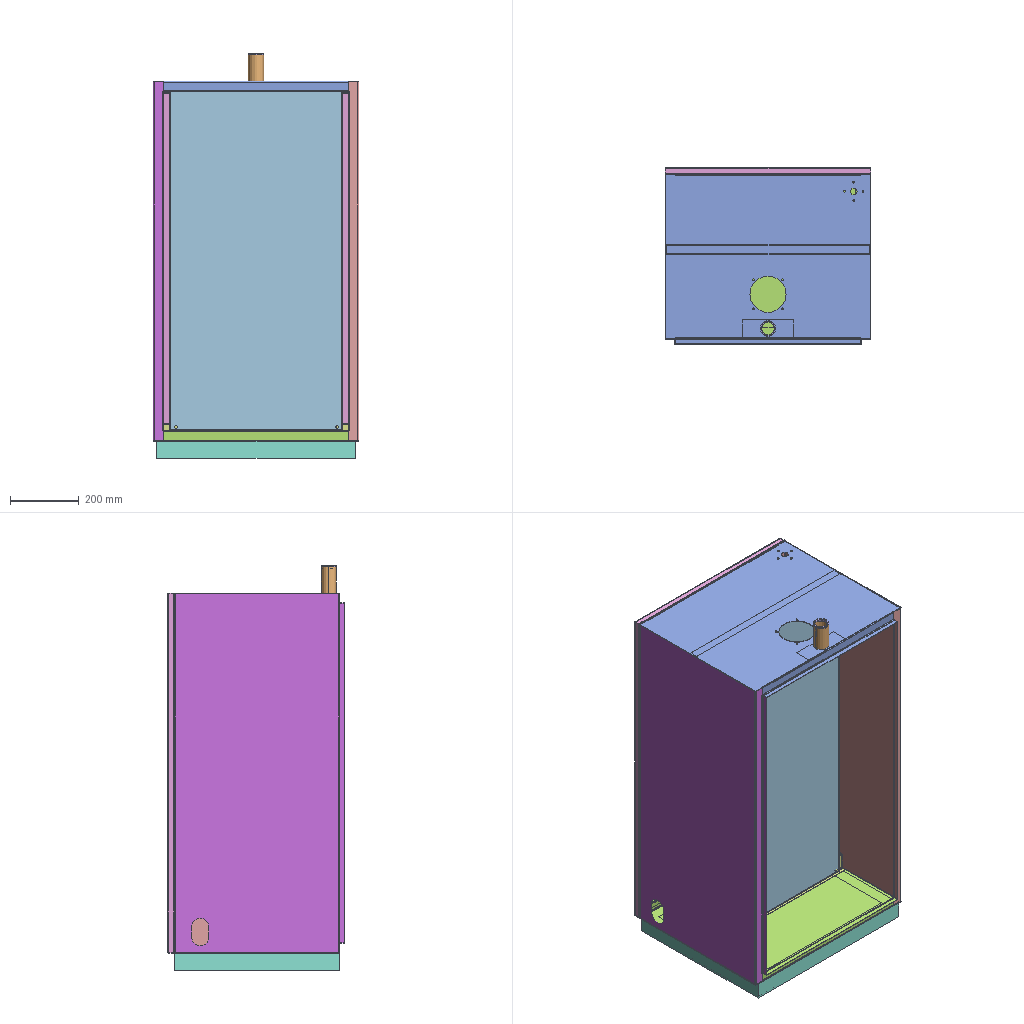Assembly | SolidWorks | 13 different items | 14 placed | box 600 x 515 x 1180 mm
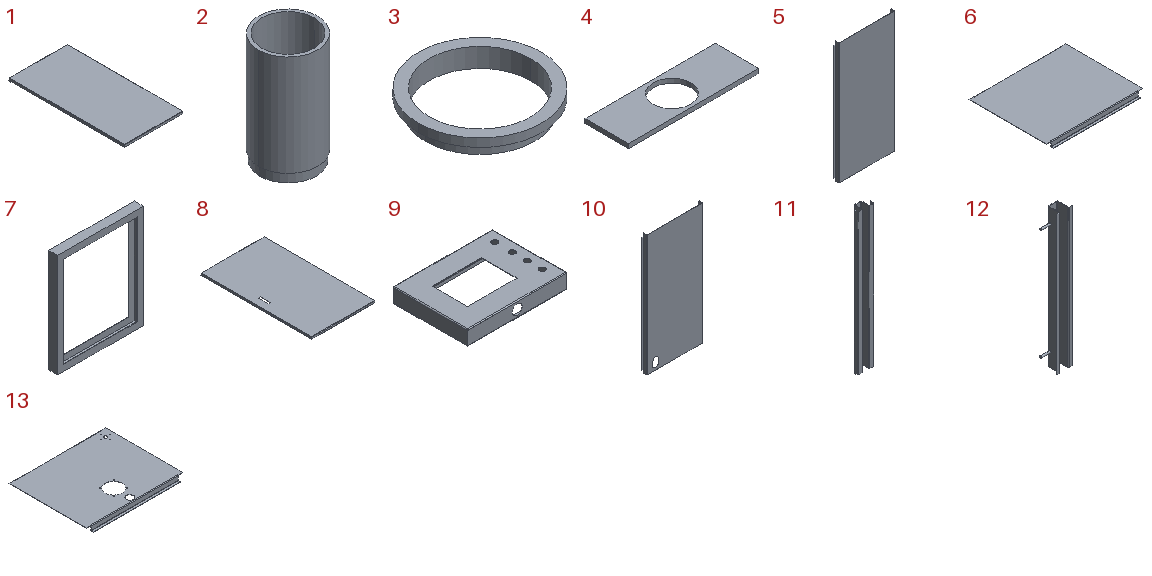Parts list (item | quantity | size | volume | features):
1 | x2 | 505 x 1000 x 25 mm | 849677 mm3 | features EdgeFlange 2, CornerFeat 1, FlatPattern 1, ICE 1, SMBaseFlange 1, SheetMetal 1
2 | x1 | 45 x 45 x 84 mm | 27071 mm3 | features Extrusion 1, ICE 1
3 | x1 | 45 x 45 x 7 mm | 2271 mm3 | features Extrusion 1, ICE 1
4 | x1 | 150 x 50 x 5 mm | 30239 mm3 | features FlatPattern 1, ICE 1, SMBaseFlange 1, SheetMetal 1
5 | x1 | 510 x 30 x 1047 mm | 882007 mm3 | features EdgeFlange 2, FlatPattern 1, SMBaseFlange 1, SheetMetal 1
6 | x1 | 600 x 510 x 30 mm | 499324 mm3 | features EdgeFlange 2, FlatPattern 1, SMBaseFlange 1, SheetMetal 1
7 | x1 | 480 x 50 x 580 mm | 907872 mm3 | features ICE 2, Extrusion 1
8 | x1 | 600 x 1050 x 20 mm | 1074617 mm3 | features EdgeFlange 2, CornerFeat 1, FlatPattern 1, ICE 1, SMBaseFlange 1, SheetMetal 1
9 | x1 | 400 x 300 x 73.5 mm | 309583 mm3 | features EdgeFlange 3, ICE 2, CornerFeat 1, FlatPattern 1, SMBaseFlange 1, SheetMetal 1
10 | x1 | 510 x 30 x 1047 mm | 876812 mm3 | features EdgeFlange 2, FlatPattern 1, ICE 1, SMBaseFlange 1, SheetMetal 1
11 | x1 | 67 x 35 x 590 mm | 137357 mm3 | features FlatPattern 1, SMBaseFlange 1, SheetMetal 1
12 | x1 | 120 x 50 x 590 mm | 149764 mm3 | features ICE 2, EdgeFlange 1, FlatPattern 1, SMBaseFlange 1, SheetMetal 1
13 | x1 | 600 x 510 x 30 mm | 483219 mm3 | features ICE 3, EdgeFlange 2, FlatPattern 1, SMBaseFlange 1, SheetMetal 1
Mates (type | each side: item.copy, entity, surface, feature):
Coincident | 5.1 face plane Base-Flange1 | 13.1 face plane Base-Flange1 | 2 times
Coincident | 5.1 face plane Edge-Flange1 | 13.1 face plane Edge-Flange1
Coincident | 5.1 face plane Base-Flange1 | 6.1 face plane Base-Flange1 | 2 times
Coincident | 5.1 face plane Edge-Flange1 | 6.1 face plane Base-Flange1
Coincident | 13.1 face plane Edge-Flange1 | 8.1 face plane Edge-Flange2
Coincident | 5.1 face plane Base-Flange1 | 8.1 face plane Edge-Flange1
Coincident | 13.1 face plane Base-Flange1 | 8.1 face plane Edge-Flange1
Coincident | 6.1 face plane Base-Flange1 | 7.1 face plane Boss-Extrude1
Coincident | 6.1 face plane Edge-Flange1 | 7.1 face plane Boss-Extrude1
DistanceDim | 7.1 face plane Boss-Extrude1 | 5.1 face plane Base-Flange1
Concentric | 13.1 face cylinder Cut-Extrude2 | 2.1 face cylinder Cut-Extrude1
Coincident | 13.1 face plane Base-Flange1 | 2.1 face plane Cut-Extrude1
Coincident | 5.1 face plane Base-Flange1 | assembly plane
Concentric | 2.1 face cylinder Boss-Extrude1 | 3.1 face cylinder Boss-Extrude2
Coincident | 2.1 face plane Boss-Extrude1 | 3.1 face plane Boss-Extrude1
Concentric | 2.1 face cylinder Cut-Extrude1 | 4.1 face cylinder Cut-Extrude1
Coincident | 13.1 face plane Base-Flange1 | 4.1 face plane Base-Flange1
Coincident | 13.1 face plane Base-Flange1 | 11.1 face plane Base-Flange1
DistanceDim | 11.1 face plane Base-Flange1 | 5.1 face plane Base-Flange1
DistanceDim | 11.1 face plane Base-Flange1 | 8.1 face plane Base-Flange1
Coincident | 11.1 face plane Base-Flange1 | 1.1 face plane Edge-Flange2
Coincident | 11.1 face plane Base-Flange1 | 1.1 face plane Edge-Flange1
Coincident | 11.1 face plane Base-Flange1 | 1.2 face plane Edge-Flange2
Coincident | 1.1 face plane Edge-Flange1 | 1.2 face plane Edge-Flange1
Coincident | 11.1 edge | 1.2 face plane Edge-Flange1
Coincident | 6.1 face plane Base-Flange1 | 12.1 face plane Edge-Flange1
Coincident | 13.1 face plane Base-Flange1 | 10.1 face plane Base-Flange1 | 2 times